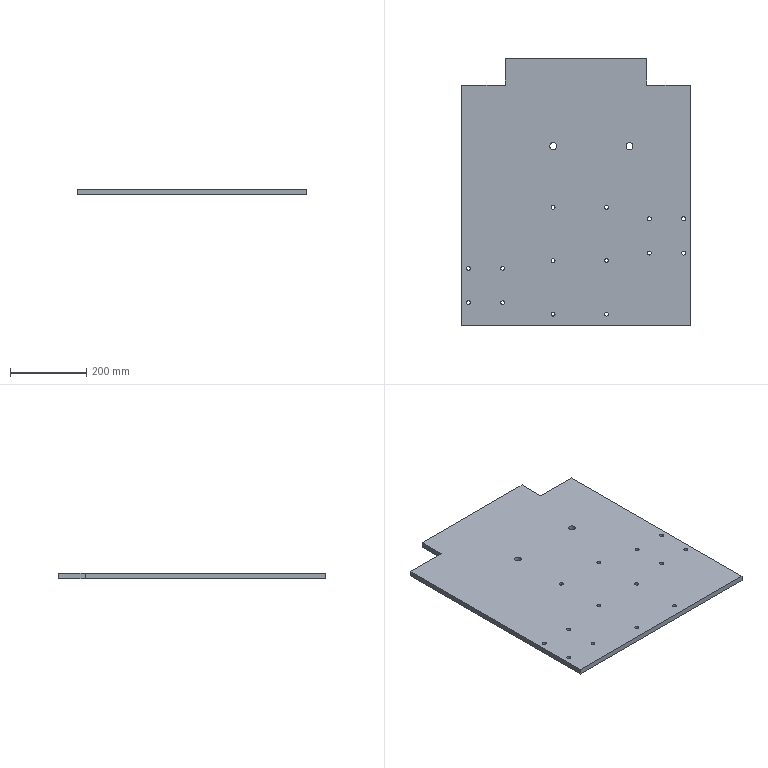Part | SolidWorks | features 3DProfileFeature 1, Extrusion 1, HoleWzd 1 | 1 solid | 42 faces | box 600 x 700 x 14 mm | volume 5631459 mm3 | cylinder 32 | plane 10 | commonest cylinder face diameters 10.2 x28 18 x4
STEP:
#1=CARTESIAN_POINT('',(12.9,150.,0.));
#2=VERTEX_POINT('',#1);
#3=CARTESIAN_POINT('',(23.1,150.,0.));
#4=VERTEX_POINT('',#3);
#5=CARTESIAN_POINT('',(18.,150.,0.));
#6=DIRECTION('',(0.,0.,1.));
#7=DIRECTION('',(1.,0.,0.));
#8=AXIS2_PLACEMENT_3D('',#5,#6,#7);
#9=CIRCLE('',#8,5.1);
#10=EDGE_CURVE('',#2,#4,#9,.T.);
#11=ORIENTED_EDGE('',*,*,#10,.F.);
#12=CARTESIAN_POINT('',(12.9,150.,14.));
#13=VERTEX_POINT('',#12);
#14=CARTESIAN_POINT('',(12.9,150.,14.));
#15=DIRECTION('',(0.,0.,1.));
#16=VECTOR('',#15,1000.);
#17=LINE('',#14,#16);
#18=EDGE_CURVE('',#2,#13,#17,.T.);
#19=ORIENTED_EDGE('',*,*,#18,.T.);
#20=CARTESIAN_POINT('',(23.1,150.,14.));
#21=VERTEX_POINT('',#20);
#22=CARTESIAN_POINT('',(18.,150.,14.));
#23=DIRECTION('',(0.,0.,1.));
#24=DIRECTION('',(1.,0.,0.));
#25=AXIS2_PLACEMENT_3D('',#22,#23,#24);
#26=CIRCLE('',#25,5.1);
#27=EDGE_CURVE('',#13,#21,#26,.T.);
#28=ORIENTED_EDGE('',*,*,#27,.T.);
#29=CARTESIAN_POINT('',(23.1,150.,14.));
#30=DIRECTION('',(0.,0.,1.));
#31=VECTOR('',#30,1000.);
#32=LINE('',#29,#31);
#33=EDGE_CURVE('',#4,#21,#32,.T.);
#34=ORIENTED_EDGE('',*,*,#33,.F.);
#35=EDGE_LOOP('',(#11,#19,#28,#34));
#36=FACE_OUTER_BOUND('',#35,.T.);
#37=CARTESIAN_POINT('',(18.,150.,14.));
#38=DIRECTION('',(0.,0.,1.));
#39=DIRECTION('',(1.,0.,0.));
#40=AXIS2_PLACEMENT_3D('',#37,#38,#39);
#41=CYLINDRICAL_SURFACE('',#40,5.1);
#42=ADVANCED_FACE('',(#36),#41,.F.);
#43=CARTESIAN_POINT('',(102.9,150.,0.));
#44=VERTEX_POINT('',#43);
#45=CARTESIAN_POINT('',(113.1,150.,0.));
#46=VERTEX_POINT('',#45);
#47=CARTESIAN_POINT('',(108.,150.,0.));
#48=DIRECTION('',(0.,0.,1.));
#49=DIRECTION('',(1.,0.,0.));
#50=AXIS2_PLACEMENT_3D('',#47,#48,#49);
#51=CIRCLE('',#50,5.1);
#52=EDGE_CURVE('',#44,#46,#51,.T.);
#53=ORIENTED_EDGE('',*,*,#52,.F.);
#54=CARTESIAN_POINT('',(102.9,150.,14.));
#55=VERTEX_POINT('',#54);
#56=CARTESIAN_POINT('',(102.9,150.,14.));
#57=DIRECTION('',(0.,0.,1.));
#58=VECTOR('',#57,1000.);
#59=LINE('',#56,#58);
#60=EDGE_CURVE('',#44,#55,#59,.T.);
#61=ORIENTED_EDGE('',*,*,#60,.T.);
#62=CARTESIAN_POINT('',(113.1,150.,14.));
#63=VERTEX_POINT('',#62);
#64=CARTESIAN_POINT('',(108.,150.,14.));
#65=DIRECTION('',(0.,0.,1.));
#66=DIRECTION('',(1.,0.,0.));
#67=AXIS2_PLACEMENT_3D('',#64,#65,#66);
#68=CIRCLE('',#67,5.1);
#69=EDGE_CURVE('',#55,#63,#68,.T.);
#70=ORIENTED_EDGE('',*,*,#69,.T.);
#71=CARTESIAN_POINT('',(113.1,150.,14.));
#72=DIRECTION('',(0.,0.,1.));
#73=VECTOR('',#72,1000.);
#74=LINE('',#71,#73);
#75=EDGE_CURVE('',#46,#63,#74,.T.);
#76=ORIENTED_EDGE('',*,*,#75,.F.);
#77=EDGE_LOOP('',(#53,#61,#70,#76));
#78=FACE_OUTER_BOUND('',#77,.T.);
#79=CARTESIAN_POINT('',(108.,150.,14.));
#80=DIRECTION('',(0.,0.,1.));
#81=DIRECTION('',(1.,0.,0.));
#82=AXIS2_PLACEMENT_3D('',#79,#80,#81);
#83=CYLINDRICAL_SURFACE('',#82,5.1);
#84=ADVANCED_FACE('',(#78),#83,.F.);
#85=CARTESIAN_POINT('',(12.9,60.,0.));
#86=VERTEX_POINT('',#85);
#87=CARTESIAN_POINT('',(23.1,60.,0.));
#88=VERTEX_POINT('',#87);
#89=CARTESIAN_POINT('',(18.,60.,0.));
#90=DIRECTION('',(0.,0.,1.));
#91=DIRECTION('',(1.,0.,0.));
#92=AXIS2_PLACEMENT_3D('',#89,#90,#91);
#93=CIRCLE('',#92,5.1);
#94=EDGE_CURVE('',#86,#88,#93,.T.);
#95=ORIENTED_EDGE('',*,*,#94,.F.);
#96=CARTESIAN_POINT('',(12.9,60.,14.));
#97=VERTEX_POINT('',#96);
#98=CARTESIAN_POINT('',(12.9,60.,14.));
#99=DIRECTION('',(0.,0.,1.));
#100=VECTOR('',#99,1000.);
#101=LINE('',#98,#100);
#102=EDGE_CURVE('',#86,#97,#101,.T.);
#103=ORIENTED_EDGE('',*,*,#102,.T.);
#104=CARTESIAN_POINT('',(23.1,60.,14.));
#105=VERTEX_POINT('',#104);
#106=CARTESIAN_POINT('',(18.,60.,14.));
#107=DIRECTION('',(0.,0.,1.));
#108=DIRECTION('',(1.,0.,0.));
#109=AXIS2_PLACEMENT_3D('',#106,#107,#108);
#110=CIRCLE('',#109,5.1);
#111=EDGE_CURVE('',#97,#105,#110,.T.);
#112=ORIENTED_EDGE('',*,*,#111,.T.);
#113=CARTESIAN_POINT('',(23.1,60.,14.));
#114=DIRECTION('',(0.,0.,1.));
#115=VECTOR('',#114,1000.);
#116=LINE('',#113,#115);
#117=EDGE_CURVE('',#88,#105,#116,.T.);
#118=ORIENTED_EDGE('',*,*,#117,.F.);
#119=EDGE_LOOP('',(#95,#103,#112,#118));
#120=FACE_OUTER_BOUND('',#119,.T.);
#121=CARTESIAN_POINT('',(18.,60.,14.));
#122=DIRECTION('',(0.,0.,1.));
#123=DIRECTION('',(1.,0.,0.));
#124=AXIS2_PLACEMENT_3D('',#121,#122,#123);
#125=CYLINDRICAL_SURFACE('',#124,5.1);
#126=ADVANCED_FACE('',(#120),#125,.F.);
#127=CARTESIAN_POINT('',(102.9,60.,0.));
#128=VERTEX_POINT('',#127);
#129=CARTESIAN_POINT('',(113.1,60.,0.));
#130=VERTEX_POINT('',#129);
#131=CARTESIAN_POINT('',(108.,60.,0.));
#132=DIRECTION('',(0.,0.,1.));
#133=DIRECTION('',(1.,0.,0.));
#134=AXIS2_PLACEMENT_3D('',#131,#132,#133);
#135=CIRCLE('',#134,5.1);
#136=EDGE_CURVE('',#128,#130,#135,.T.);
#137=ORIENTED_EDGE('',*,*,#136,.F.);
#138=CARTESIAN_POINT('',(102.9,60.,14.));
#139=VERTEX_POINT('',#138);
#140=CARTESIAN_POINT('',(102.9,60.,14.));
#141=DIRECTION('',(0.,0.,1.));
#142=VECTOR('',#141,1000.);
#143=LINE('',#140,#142);
#144=EDGE_CURVE('',#128,#139,#143,.T.);
#145=ORIENTED_EDGE('',*,*,#144,.T.);
#146=CARTESIAN_POINT('',(113.1,60.,14.));
#147=VERTEX_POINT('',#146);
#148=CARTESIAN_POINT('',(108.,60.,14.));
#149=DIRECTION('',(0.,0.,1.));
#150=DIRECTION('',(1.,0.,0.));
#151=AXIS2_PLACEMENT_3D('',#148,#149,#150);
#152=CIRCLE('',#151,5.1);
#153=EDGE_CURVE('',#139,#147,#152,.T.);
#154=ORIENTED_EDGE('',*,*,#153,.T.);
#155=CARTESIAN_POINT('',(113.1,60.,14.));
#156=DIRECTION('',(0.,0.,1.));
#157=VECTOR('',#156,1000.);
#158=LINE('',#155,#157);
#159=EDGE_CURVE('',#130,#147,#158,.T.);
#160=ORIENTED_EDGE('',*,*,#159,.F.);
#161=EDGE_LOOP('',(#137,#145,#154,#160));
#162=FACE_OUTER_BOUND('',#161,.T.);
#163=CARTESIAN_POINT('',(108.,60.,14.));
#164=DIRECTION('',(0.,0.,1.));
#165=DIRECTION('',(1.,0.,0.));
#166=AXIS2_PLACEMENT_3D('',#163,#164,#165);
#167=CYLINDRICAL_SURFACE('',#166,5.1);
#168=ADVANCED_FACE('',(#162),#167,.F.);
#169=CARTESIAN_POINT('',(486.9,280.,0.));
#170=VERTEX_POINT('',#169);
#171=CARTESIAN_POINT('',(497.1,280.,0.));
#172=VERTEX_POINT('',#171);
#173=CARTESIAN_POINT('',(492.,280.,0.));
#174=DIRECTION('',(0.,0.,1.));
#175=DIRECTION('',(1.,0.,0.));
#176=AXIS2_PLACEMENT_3D('',#173,#174,#175);
#177=CIRCLE('',#176,5.1);
#178=EDGE_CURVE('',#170,#172,#177,.T.);
#179=ORIENTED_EDGE('',*,*,#178,.F.);
#180=CARTESIAN_POINT('',(486.9,280.,14.));
#181=VERTEX_POINT('',#180);
#182=CARTESIAN_POINT('',(486.9,280.,14.));
#183=DIRECTION('',(0.,0.,1.));
#184=VECTOR('',#183,1000.);
#185=LINE('',#182,#184);
#186=EDGE_CURVE('',#170,#181,#185,.T.);
#187=ORIENTED_EDGE('',*,*,#186,.T.);
#188=CARTESIAN_POINT('',(497.1,280.,14.));
#189=VERTEX_POINT('',#188);
#190=CARTESIAN_POINT('',(492.,280.,14.));
#191=DIRECTION('',(0.,0.,1.));
#192=DIRECTION('',(1.,0.,0.));
#193=AXIS2_PLACEMENT_3D('',#190,#191,#192);
#194=CIRCLE('',#193,5.1);
#195=EDGE_CURVE('',#181,#189,#194,.T.);
#196=ORIENTED_EDGE('',*,*,#195,.T.);
#197=CARTESIAN_POINT('',(497.1,280.,14.));
#198=DIRECTION('',(0.,0.,1.));
#199=VECTOR('',#198,1000.);
#200=LINE('',#197,#199);
#201=EDGE_CURVE('',#172,#189,#200,.T.);
#202=ORIENTED_EDGE('',*,*,#201,.F.);
#203=EDGE_LOOP('',(#179,#187,#196,#202));
#204=FACE_OUTER_BOUND('',#203,.T.);
#205=CARTESIAN_POINT('',(492.,280.,14.));
#206=DIRECTION('',(0.,0.,1.));
#207=DIRECTION('',(1.,0.,0.));
#208=AXIS2_PLACEMENT_3D('',#205,#206,#207);
#209=CYLINDRICAL_SURFACE('',#208,5.1);
#210=ADVANCED_FACE('',(#204),#209,.F.);
#211=CARTESIAN_POINT('',(576.9,280.,0.));
#212=VERTEX_POINT('',#211);
#213=CARTESIAN_POINT('',(587.1,280.,0.));
#214=VERTEX_POINT('',#213);
#215=CARTESIAN_POINT('',(582.,280.,0.));
#216=DIRECTION('',(0.,0.,1.));
#217=DIRECTION('',(1.,0.,0.));
#218=AXIS2_PLACEMENT_3D('',#215,#216,#217);
#219=CIRCLE('',#218,5.1);
#220=EDGE_CURVE('',#212,#214,#219,.T.);
#221=ORIENTED_EDGE('',*,*,#220,.F.);
#222=CARTESIAN_POINT('',(576.9,280.,14.));
#223=VERTEX_POINT('',#222);
#224=CARTESIAN_POINT('',(576.9,280.,14.));
#225=DIRECTION('',(0.,0.,1.));
#226=VECTOR('',#225,1000.);
#227=LINE('',#224,#226);
#228=EDGE_CURVE('',#212,#223,#227,.T.);
#229=ORIENTED_EDGE('',*,*,#228,.T.);
#230=CARTESIAN_POINT('',(587.1,280.,14.));
#231=VERTEX_POINT('',#230);
#232=CARTESIAN_POINT('',(582.,280.,14.));
#233=DIRECTION('',(0.,0.,1.));
#234=DIRECTION('',(1.,0.,0.));
#235=AXIS2_PLACEMENT_3D('',#232,#233,#234);
#236=CIRCLE('',#235,5.1);
#237=EDGE_CURVE('',#223,#231,#236,.T.);
#238=ORIENTED_EDGE('',*,*,#237,.T.);
#239=CARTESIAN_POINT('',(587.1,280.,14.));
#240=DIRECTION('',(0.,0.,1.));
#241=VECTOR('',#240,1000.);
#242=LINE('',#239,#241);
#243=EDGE_CURVE('',#214,#231,#242,.T.);
#244=ORIENTED_EDGE('',*,*,#243,.F.);
#245=EDGE_LOOP('',(#221,#229,#238,#244));
#246=FACE_OUTER_BOUND('',#245,.T.);
#247=CARTESIAN_POINT('',(582.,280.,14.));
#248=DIRECTION('',(0.,0.,1.));
#249=DIRECTION('',(1.,0.,0.));
#250=AXIS2_PLACEMENT_3D('',#247,#248,#249);
#251=CYLINDRICAL_SURFACE('',#250,5.1);
#252=ADVANCED_FACE('',(#246),#251,.F.);
#253=CARTESIAN_POINT('',(486.9,190.,0.));
#254=VERTEX_POINT('',#253);
#255=CARTESIAN_POINT('',(497.1,190.,0.));
#256=VERTEX_POINT('',#255);
#257=CARTESIAN_POINT('',(492.,190.,0.));
#258=DIRECTION('',(0.,0.,1.));
#259=DIRECTION('',(1.,0.,0.));
#260=AXIS2_PLACEMENT_3D('',#257,#258,#259);
#261=CIRCLE('',#260,5.1);
#262=EDGE_CURVE('',#254,#256,#261,.T.);
#263=ORIENTED_EDGE('',*,*,#262,.F.);
#264=CARTESIAN_POINT('',(486.9,190.,14.));
#265=VERTEX_POINT('',#264);
#266=CARTESIAN_POINT('',(486.9,190.,14.));
#267=DIRECTION('',(0.,0.,1.));
#268=VECTOR('',#267,1000.);
#269=LINE('',#266,#268);
#270=EDGE_CURVE('',#254,#265,#269,.T.);
#271=ORIENTED_EDGE('',*,*,#270,.T.);
#272=CARTESIAN_POINT('',(497.1,190.,14.));
#273=VERTEX_POINT('',#272);
#274=CARTESIAN_POINT('',(492.,190.,14.));
#275=DIRECTION('',(0.,0.,1.));
#276=DIRECTION('',(1.,0.,0.));
#277=AXIS2_PLACEMENT_3D('',#274,#275,#276);
#278=CIRCLE('',#277,5.1);
#279=EDGE_CURVE('',#265,#273,#278,.T.);
#280=ORIENTED_EDGE('',*,*,#279,.T.);
#281=CARTESIAN_POINT('',(497.1,190.,14.));
#282=DIRECTION('',(0.,0.,1.));
#283=VECTOR('',#282,1000.);
#284=LINE('',#281,#283);
#285=EDGE_CURVE('',#256,#273,#284,.T.);
#286=ORIENTED_EDGE('',*,*,#285,.F.);
#287=EDGE_LOOP('',(#263,#271,#280,#286));
#288=FACE_OUTER_BOUND('',#287,.T.);
#289=CARTESIAN_POINT('',(492.,190.,14.));
#290=DIRECTION('',(0.,0.,1.));
#291=DIRECTION('',(1.,0.,0.));
#292=AXIS2_PLACEMENT_3D('',#289,#290,#291);
#293=CYLINDRICAL_SURFACE('',#292,5.1);
#294=ADVANCED_FACE('',(#288),#293,.F.);
#295=CARTESIAN_POINT('',(576.9,190.,0.));
#296=VERTEX_POINT('',#295);
#297=CARTESIAN_POINT('',(587.1,190.,0.));
#298=VERTEX_POINT('',#297);
#299=CARTESIAN_POINT('',(582.,190.,0.));
#300=DIRECTION('',(0.,0.,1.));
#301=DIRECTION('',(1.,0.,0.));
#302=AXIS2_PLACEMENT_3D('',#299,#300,#301);
#303=CIRCLE('',#302,5.1);
#304=EDGE_CURVE('',#296,#298,#303,.T.);
#305=ORIENTED_EDGE('',*,*,#304,.F.);
#306=CARTESIAN_POINT('',(576.9,190.,14.));
#307=VERTEX_POINT('',#306);
#308=CARTESIAN_POINT('',(576.9,190.,14.));
#309=DIRECTION('',(0.,0.,1.));
#310=VECTOR('',#309,1000.);
#311=LINE('',#308,#310);
#312=EDGE_CURVE('',#296,#307,#311,.T.);
#313=ORIENTED_EDGE('',*,*,#312,.T.);
#314=CARTESIAN_POINT('',(587.1,190.,14.));
#315=VERTEX_POINT('',#314);
#316=CARTESIAN_POINT('',(582.,190.,14.));
#317=DIRECTION('',(0.,0.,1.));
#318=DIRECTION('',(1.,0.,0.));
#319=AXIS2_PLACEMENT_3D('',#316,#317,#318);
#320=CIRCLE('',#319,5.1);
#321=EDGE_CURVE('',#307,#315,#320,.T.);
#322=ORIENTED_EDGE('',*,*,#321,.T.);
#323=CARTESIAN_POINT('',(587.1,190.,14.));
#324=DIRECTION('',(0.,0.,1.));
#325=VECTOR('',#324,1000.);
#326=LINE('',#323,#325);
#327=EDGE_CURVE('',#298,#315,#326,.T.);
#328=ORIENTED_EDGE('',*,*,#327,.F.);
#329=EDGE_LOOP('',(#305,#313,#322,#328));
#330=FACE_OUTER_BOUND('',#329,.T.);
#331=CARTESIAN_POINT('',(582.,190.,14.));
#332=DIRECTION('',(0.,0.,1.));
#333=DIRECTION('',(1.,0.,0.));
#334=AXIS2_PLACEMENT_3D('',#331,#332,#333);
#335=CYLINDRICAL_SURFACE('',#334,5.1);
#336=ADVANCED_FACE('',(#330),#335,.F.);
#337=CARTESIAN_POINT('',(234.9,310.,0.));
#338=VERTEX_POINT('',#337);
#339=CARTESIAN_POINT('',(245.1,310.,0.));
#340=VERTEX_POINT('',#339);
#341=CARTESIAN_POINT('',(240.,310.,0.));
#342=DIRECTION('',(0.,0.,1.));
#343=DIRECTION('',(1.,0.,0.));
#344=AXIS2_PLACEMENT_3D('',#341,#342,#343);
#345=CIRCLE('',#344,5.1);
#346=EDGE_CURVE('',#338,#340,#345,.T.);
#347=ORIENTED_EDGE('',*,*,#346,.F.);
#348=CARTESIAN_POINT('',(234.9,310.,14.));
#349=VERTEX_POINT('',#348);
#350=CARTESIAN_POINT('',(234.9,310.,14.));
#351=DIRECTION('',(0.,0.,1.));
#352=VECTOR('',#351,1000.);
#353=LINE('',#350,#352);
#354=EDGE_CURVE('',#338,#349,#353,.T.);
#355=ORIENTED_EDGE('',*,*,#354,.T.);
#356=CARTESIAN_POINT('',(245.1,310.,14.));
#357=VERTEX_POINT('',#356);
#358=CARTESIAN_POINT('',(240.,310.,14.));
#359=DIRECTION('',(0.,0.,1.));
#360=DIRECTION('',(1.,0.,0.));
#361=AXIS2_PLACEMENT_3D('',#358,#359,#360);
#362=CIRCLE('',#361,5.1);
#363=EDGE_CURVE('',#349,#357,#362,.T.);
#364=ORIENTED_EDGE('',*,*,#363,.T.);
#365=CARTESIAN_POINT('',(245.1,310.,14.));
#366=DIRECTION('',(0.,0.,1.));
#367=VECTOR('',#366,1000.);
#368=LINE('',#365,#367);
#369=EDGE_CURVE('',#340,#357,#368,.T.);
#370=ORIENTED_EDGE('',*,*,#369,.F.);
#371=EDGE_LOOP('',(#347,#355,#364,#370));
#372=FACE_OUTER_BOUND('',#371,.T.);
#373=CARTESIAN_POINT('',(240.,310.,14.));
#374=DIRECTION('',(0.,0.,1.));
#375=DIRECTION('',(1.,0.,0.));
#376=AXIS2_PLACEMENT_3D('',#373,#374,#375);
#377=CYLINDRICAL_SURFACE('',#376,5.1);
#378=ADVANCED_FACE('',(#372),#377,.F.);
#379=CARTESIAN_POINT('',(374.9,310.,0.));
#380=VERTEX_POINT('',#379);
#381=CARTESIAN_POINT('',(385.1,310.,0.));
#382=VERTEX_POINT('',#381);
#383=CARTESIAN_POINT('',(380.,310.,0.));
#384=DIRECTION('',(0.,0.,1.));
#385=DIRECTION('',(1.,0.,0.));
#386=AXIS2_PLACEMENT_3D('',#383,#384,#385);
#387=CIRCLE('',#386,5.1);
#388=EDGE_CURVE('',#380,#382,#387,.T.);
#389=ORIENTED_EDGE('',*,*,#388,.F.);
#390=CARTESIAN_POINT('',(374.9,310.,14.));
#391=VERTEX_POINT('',#390);
#392=CARTESIAN_POINT('',(374.9,310.,14.));
#393=DIRECTION('',(0.,0.,1.));
#394=VECTOR('',#393,1000.);
#395=LINE('',#392,#394);
#396=EDGE_CURVE('',#380,#391,#395,.T.);
#397=ORIENTED_EDGE('',*,*,#396,.T.);
#398=CARTESIAN_POINT('',(385.1,310.,14.));
#399=VERTEX_POINT('',#398);
#400=CARTESIAN_POINT('',(380.,310.,14.));
#401=DIRECTION('',(0.,0.,1.));
#402=DIRECTION('',(1.,0.,0.));
#403=AXIS2_PLACEMENT_3D('',#400,#401,#402);
#404=CIRCLE('',#403,5.1);
#405=EDGE_CURVE('',#391,#399,#404,.T.);
#406=ORIENTED_EDGE('',*,*,#405,.T.);
#407=CARTESIAN_POINT('',(385.1,310.,14.));
#408=DIRECTION('',(0.,0.,1.));
#409=VECTOR('',#408,1000.);
#410=LINE('',#407,#409);
#411=EDGE_CURVE('',#382,#399,#410,.T.);
#412=ORIENTED_EDGE('',*,*,#411,.F.);
#413=EDGE_LOOP('',(#389,#397,#406,#412));
#414=FACE_OUTER_BOUND('',#413,.T.);
#415=CARTESIAN_POINT('',(380.,310.,14.));
#416=DIRECTION('',(0.,0.,1.));
#417=DIRECTION('',(1.,0.,0.));
#418=AXIS2_PLACEMENT_3D('',#415,#416,#417);
#419=CYLINDRICAL_SURFACE('',#418,5.1);
#420=ADVANCED_FACE('',(#414),#419,.F.);
#421=CARTESIAN_POINT('',(234.9,170.,0.));
#422=VERTEX_POINT('',#421);
#423=CARTESIAN_POINT('',(245.1,170.,0.));
#424=VERTEX_POINT('',#423);
#425=CARTESIAN_POINT('',(240.,170.,0.));
#426=DIRECTION('',(0.,0.,1.));
#427=DIRECTION('',(1.,0.,0.));
#428=AXIS2_PLACEMENT_3D('',#425,#426,#427);
#429=CIRCLE('',#428,5.1);
#430=EDGE_CURVE('',#422,#424,#429,.T.);
#431=ORIENTED_EDGE('',*,*,#430,.F.);
#432=CARTESIAN_POINT('',(234.9,170.,14.));
#433=VERTEX_POINT('',#432);
#434=CARTESIAN_POINT('',(234.9,170.,14.));
#435=DIRECTION('',(0.,0.,1.));
#436=VECTOR('',#435,1000.);
#437=LINE('',#434,#436);
#438=EDGE_CURVE('',#422,#433,#437,.T.);
#439=ORIENTED_EDGE('',*,*,#438,.T.);
#440=CARTESIAN_POINT('',(245.1,170.,14.));
#441=VERTEX_POINT('',#440);
#442=CARTESIAN_POINT('',(240.,170.,14.));
#443=DIRECTION('',(0.,0.,1.));
#444=DIRECTION('',(1.,0.,0.));
#445=AXIS2_PLACEMENT_3D('',#442,#443,#444);
#446=CIRCLE('',#445,5.1);
#447=EDGE_CURVE('',#433,#441,#446,.T.);
#448=ORIENTED_EDGE('',*,*,#447,.T.);
#449=CARTESIAN_POINT('',(245.1,170.,14.));
#450=DIRECTION('',(0.,0.,1.));
#451=VECTOR('',#450,1000.);
#452=LINE('',#449,#451);
#453=EDGE_CURVE('',#424,#441,#452,.T.);
#454=ORIENTED_EDGE('',*,*,#453,.F.);
#455=EDGE_LOOP('',(#431,#439,#448,#454));
#456=FACE_OUTER_BOUND('',#455,.T.);
#457=CARTESIAN_POINT('',(240.,170.,14.));
#458=DIRECTION('',(0.,0.,1.));
#459=DIRECTION('',(1.,0.,0.));
#460=AXIS2_PLACEMENT_3D('',#457,#458,#459);
#461=CYLINDRICAL_SURFACE('',#460,5.1);
#462=ADVANCED_FACE('',(#456),#461,.F.);
#463=CARTESIAN_POINT('',(374.9,170.,0.));
#464=VERTEX_POINT('',#463);
#465=CARTESIAN_POINT('',(385.1,170.,0.));
#466=VERTEX_POINT('',#465);
#467=CARTESIAN_POINT('',(380.,170.,0.));
#468=DIRECTION('',(0.,0.,1.));
#469=DIRECTION('',(1.,0.,0.));
#470=AXIS2_PLACEMENT_3D('',#467,#468,#469);
#471=CIRCLE('',#470,5.1);
#472=EDGE_CURVE('',#464,#466,#471,.T.);
#473=ORIENTED_EDGE('',*,*,#472,.F.);
#474=CARTESIAN_POINT('',(374.9,170.,14.));
#475=VERTEX_POINT('',#474);
#476=CARTESIAN_POINT('',(374.9,170.,14.));
#477=DIRECTION('',(0.,0.,1.));
#478=VECTOR('',#477,1000.);
#479=LINE('',#476,#478);
#480=EDGE_CURVE('',#464,#475,#479,.T.);
#481=ORIENTED_EDGE('',*,*,#480,.T.);
#482=CARTESIAN_POINT('',(385.1,170.,14.));
#483=VERTEX_POINT('',#482);
#484=CARTESIAN_POINT('',(380.,170.,14.));
#485=DIRECTION('',(0.,0.,1.));
#486=DIRECTION('',(1.,0.,0.));
#487=AXIS2_PLACEMENT_3D('',#484,#485,#486);
#488=CIRCLE('',#487,5.1);
#489=EDGE_CURVE('',#475,#483,#488,.T.);
#490=ORIENTED_EDGE('',*,*,#489,.T.);
#491=CARTESIAN_POINT('',(385.1,170.,14.));
#492=DIRECTION('',(0.,0.,1.));
#493=VECTOR('',#492,1000.);
#494=LINE('',#491,#493);
#495=EDGE_CURVE('',#466,#483,#494,.T.);
#496=ORIENTED_EDGE('',*,*,#495,.F.);
#497=EDGE_LOOP('',(#473,#481,#490,#496));
#498=FACE_OUTER_BOUND('',#497,.T.);
#499=CARTESIAN_POINT('',(380.,170.,14.));
#500=DIRECTION('',(0.,0.,1.));
#501=DIRECTION('',(1.,0.,0.));
#502=AXIS2_PLACEMENT_3D('',#499,#500,#501);
#503=CYLINDRICAL_SURFACE('',#502,5.1);
#504=ADVANCED_FACE('',(#498),#503,.F.);
#505=CARTESIAN_POINT('',(234.9,30.,0.));
#506=VERTEX_POINT('',#505);
#507=CARTESIAN_POINT('',(245.1,30.,0.));
#508=VERTEX_POINT('',#507);
#509=CARTESIAN_POINT('',(240.,30.,0.));
#510=DIRECTION('',(0.,0.,1.));
#511=DIRECTION('',(1.,0.,0.));
#512=AXIS2_PLACEMENT_3D('',#509,#510,#511);
#513=CIRCLE('',#512,5.1);
#514=EDGE_CURVE('',#506,#508,#513,.T.);
#515=ORIENTED_EDGE('',*,*,#514,.F.);
#516=CARTESIAN_POINT('',(234.9,30.,14.));
#517=VERTEX_POINT('',#516);
#518=CARTESIAN_POINT('',(234.9,30.,14.));
#519=DIRECTION('',(0.,0.,1.));
#520=VECTOR('',#519,1000.);
#521=LINE('',#518,#520);
#522=EDGE_CURVE('',#506,#517,#521,.T.);
#523=ORIENTED_EDGE('',*,*,#522,.T.);
#524=CARTESIAN_POINT('',(245.1,30.,14.));
#525=VERTEX_POINT('',#524);
#526=CARTESIAN_POINT('',(240.,30.,14.));
#527=DIRECTION('',(0.,0.,1.));
#528=DIRECTION('',(1.,0.,0.));
#529=AXIS2_PLACEMENT_3D('',#526,#527,#528);
#530=CIRCLE('',#529,5.1);
#531=EDGE_CURVE('',#517,#525,#530,.T.);
#532=ORIENTED_EDGE('',*,*,#531,.T.);
#533=CARTESIAN_POINT('',(245.1,30.,14.));
#534=DIRECTION('',(0.,0.,1.));
#535=VECTOR('',#534,1000.);
#536=LINE('',#533,#535);
#537=EDGE_CURVE('',#508,#525,#536,.T.);
#538=ORIENTED_EDGE('',*,*,#537,.F.);
#539=EDGE_LOOP('',(#515,#523,#532,#538));
#540=FACE_OUTER_BOUND('',#539,.T.);
#541=CARTESIAN_POINT('',(240.,30.,14.));
#542=DIRECTION('',(0.,0.,1.));
#543=DIRECTION('',(1.,0.,0.));
#544=AXIS2_PLACEMENT_3D('',#541,#542,#543);
#545=CYLINDRICAL_SURFACE('',#544,5.1);
#546=ADVANCED_FACE('',(#540),#545,.F.);
#547=CARTESIAN_POINT('',(374.9,30.,0.));
#548=VERTEX_POINT('',#547);
#549=CARTESIAN_POINT('',(385.1,30.,0.));
#550=VERTEX_POINT('',#549);
#551=CARTESIAN_POINT('',(380.,30.,0.));
#552=DIRECTION('',(0.,0.,1.));
#553=DIRECTION('',(1.,0.,0.));
#554=AXIS2_PLACEMENT_3D('',#551,#552,#553);
#555=CIRCLE('',#554,5.1);
#556=EDGE_CURVE('',#548,#550,#555,.T.);
#557=ORIENTED_EDGE('',*,*,#556,.F.);
#558=CARTESIAN_POINT('',(374.9,30.,14.));
#559=VERTEX_POINT('',#558);
#560=CARTESIAN_POINT('',(374.9,30.,14.));
#561=DIRECTION('',(0.,0.,1.));
#562=VECTOR('',#561,1000.);
#563=LINE('',#560,#562);
#564=EDGE_CURVE('',#548,#559,#563,.T.);
#565=ORIENTED_EDGE('',*,*,#564,.T.);
#566=CARTESIAN_POINT('',(385.1,30.,14.));
#567=VERTEX_POINT('',#566);
#568=CARTESIAN_POINT('',(380.,30.,14.));
#569=DIRECTION('',(0.,0.,1.));
#570=DIRECTION('',(1.,0.,0.));
#571=AXIS2_PLACEMENT_3D('',#568,#569,#570);
#572=CIRCLE('',#571,5.1);
#573=EDGE_CURVE('',#559,#567,#572,.T.);
#574=ORIENTED_EDGE('',*,*,#573,.T.);
#575=CARTESIAN_POINT('',(385.1,30.,14.));
#576=DIRECTION('',(0.,0.,1.));
#577=VECTOR('',#576,1000.);
#578=LINE('',#575,#577);
#579=EDGE_CURVE('',#550,#567,#578,.T.);
#580=ORIENTED_EDGE('',*,*,#579,.F.);
#581=EDGE_LOOP('',(#557,#565,#574,#580));
#582=FACE_OUTER_BOUND('',#581,.T.);
#583=CARTESIAN_POINT('',(380.,30.,14.));
#584=DIRECTION('',(0.,0.,1.));
#585=DIRECTION('',(1.,0.,0.));
#586=AXIS2_PLACEMENT_3D('',#583,#584,#585);
#587=CYLINDRICAL_SURFACE('',#586,5.1);
#588=ADVANCED_FACE('',(#582),#587,.F.);
#589=CARTESIAN_POINT('',(231.,470.,14.));
#590=VERTEX_POINT('',#589);
#591=CARTESIAN_POINT('',(249.,470.,14.));
#592=VERTEX_POINT('',#591);
#593=CARTESIAN_POINT('',(240.,470.,14.));
#594=DIRECTION('',(0.,0.,1.));
#595=DIRECTION('',(1.,0.,0.));
#596=AXIS2_PLACEMENT_3D('',#593,#594,#595);
#597=CIRCLE('',#596,9.);
#598=EDGE_CURVE('',#590,#592,#597,.T.);
#599=ORIENTED_EDGE('',*,*,#598,.T.);
#600=CARTESIAN_POINT('',(249.,470.,0.));
#601=VERTEX_POINT('',#600);
#602=CARTESIAN_POINT('',(249.,470.,14.));
#603=DIRECTION('',(0.,0.,-1.));
#604=VECTOR('',#603,1000.);
#605=LINE('',#602,#604);
#606=EDGE_CURVE('',#592,#601,#605,.T.);
#607=ORIENTED_EDGE('',*,*,#606,.T.);
#608=CARTESIAN_POINT('',(231.,470.,0.));
#609=VERTEX_POINT('',#608);
#610=CARTESIAN_POINT('',(240.,470.,0.));
#611=DIRECTION('',(0.,0.,1.));
#612=DIRECTION('',(1.,0.,0.));
#613=AXIS2_PLACEMENT_3D('',#610,#611,#612);
#614=CIRCLE('',#613,9.);
#615=EDGE_CURVE('',#609,#601,#614,.T.);
#616=ORIENTED_EDGE('',*,*,#615,.F.);
#617=CARTESIAN_POINT('',(231.,470.,14.));
#618=DIRECTION('',(0.,0.,-1.));
#619=VECTOR('',#618,1000.);
#620=LINE('',#617,#619);
#621=EDGE_CURVE('',#590,#609,#620,.T.);
#622=ORIENTED_EDGE('',*,*,#621,.F.);
#623=EDGE_LOOP('',(#599,#607,#616,#622));
#624=FACE_OUTER_BOUND('',#623,.T.);
#625=CARTESIAN_POINT('',(240.,470.,14.));
#626=DIRECTION('',(0.,0.,-1.));
#627=DIRECTION('',(-1.,0.,0.));
#628=AXIS2_PLACEMENT_3D('',#625,#626,#627);
#629=CYLINDRICAL_SURFACE('',#628,9.);
#630=ADVANCED_FACE('',(#624),#629,.F.);
#631=CARTESIAN_POINT('',(431.,470.,14.));
#632=VERTEX_POINT('',#631);
#633=CARTESIAN_POINT('',(449.,470.,14.));
#634=VERTEX_POINT('',#633);
#635=CARTESIAN_POINT('',(440.,470.,14.));
#636=DIRECTION('',(0.,0.,1.));
#637=DIRECTION('',(1.,0.,0.));
#638=AXIS2_PLACEMENT_3D('',#635,#636,#637);
#639=CIRCLE('',#638,9.);
#640=EDGE_CURVE('',#632,#634,#639,.T.);
#641=ORIENTED_EDGE('',*,*,#640,.T.);
#642=CARTESIAN_POINT('',(449.,470.,0.));
#643=VERTEX_POINT('',#642);
#644=CARTESIAN_POINT('',(449.,470.,14.));
#645=DIRECTION('',(0.,0.,-1.));
#646=VECTOR('',#645,1000.);
#647=LINE('',#644,#646);
#648=EDGE_CURVE('',#634,#643,#647,.T.);
#649=ORIENTED_EDGE('',*,*,#648,.T.);
#650=CARTESIAN_POINT('',(431.,470.,0.));
#651=VERTEX_POINT('',#650);
#652=CARTESIAN_POINT('',(440.,470.,0.));
#653=DIRECTION('',(0.,0.,1.));
#654=DIRECTION('',(1.,0.,0.));
#655=AXIS2_PLACEMENT_3D('',#652,#653,#654);
#656=CIRCLE('',#655,9.);
#657=EDGE_CURVE('',#651,#643,#656,.T.);
#658=ORIENTED_EDGE('',*,*,#657,.F.);
#659=CARTESIAN_POINT('',(431.,470.,14.));
#660=DIRECTION('',(0.,0.,-1.));
#661=VECTOR('',#660,1000.);
#662=LINE('',#659,#661);
#663=EDGE_CURVE('',#632,#651,#662,.T.);
#664=ORIENTED_EDGE('',*,*,#663,.F.);
#665=EDGE_LOOP('',(#641,#649,#658,#664));
#666=FACE_OUTER_BOUND('',#665,.T.);
#667=CARTESIAN_POINT('',(440.,470.,14.));
#668=DIRECTION('',(0.,0.,-1.));
#669=DIRECTION('',(-1.,0.,0.));
#670=AXIS2_PLACEMENT_3D('',#667,#668,#669);
#671=CYLINDRICAL_SURFACE('',#670,9.);
#672=ADVANCED_FACE('',(#666),#671,.F.);
#673=CARTESIAN_POINT('',(18.,150.,14.));
#674=DIRECTION('',(0.,0.,1.));
#675=DIRECTION('',(1.,0.,0.));
#676=AXIS2_PLACEMENT_3D('',#673,#674,#675);
#677=CIRCLE('',#676,5.1);
#678=EDGE_CURVE('',#21,#13,#677,.T.);
#679=ORIENTED_EDGE('',*,*,#678,.F.);
#680=ORIENTED_EDGE('',*,*,#27,.F.);
#681=EDGE_LOOP('',(#679,#680));
#682=FACE_BOUND('',#681,.T.);
#683=CARTESIAN_POINT('',(108.,150.,14.));
#684=DIRECTION('',(0.,0.,1.));
#685=DIRECTION('',(1.,0.,0.));
#686=AXIS2_PLACEMENT_3D('',#683,#684,#685);
#687=CIRCLE('',#686,5.1);
#688=EDGE_CURVE('',#63,#55,#687,.T.);
#689=ORIENTED_EDGE('',*,*,#688,.F.);
#690=ORIENTED_EDGE('',*,*,#69,.F.);
#691=EDGE_LOOP('',(#689,#690));
#692=FACE_BOUND('',#691,.T.);
#693=CARTESIAN_POINT('',(18.,60.,14.));
#694=DIRECTION('',(0.,0.,1.));
#695=DIRECTION('',(1.,0.,0.));
#696=AXIS2_PLACEMENT_3D('',#693,#694,#695);
#697=CIRCLE('',#696,5.1);
#698=EDGE_CURVE('',#105,#97,#697,.T.);
#699=ORIENTED_EDGE('',*,*,#698,.F.);
#700=ORIENTED_EDGE('',*,*,#111,.F.);
#701=EDGE_LOOP('',(#699,#700));
#702=FACE_BOUND('',#701,.T.);
#703=CARTESIAN_POINT('',(108.,60.,14.));
#704=DIRECTION('',(0.,0.,1.));
#705=DIRECTION('',(1.,0.,0.));
#706=AXIS2_PLACEMENT_3D('',#703,#704,#705);
#707=CIRCLE('',#706,5.1);
#708=EDGE_CURVE('',#147,#139,#707,.T.);
#709=ORIENTED_EDGE('',*,*,#708,.F.);
#710=ORIENTED_EDGE('',*,*,#153,.F.);
#711=EDGE_LOOP('',(#709,#710));
#712=FACE_BOUND('',#711,.T.);
#713=CARTESIAN_POINT('',(492.,280.,14.));
#714=DIRECTION('',(0.,0.,1.));
#715=DIRECTION('',(1.,0.,0.));
#716=AXIS2_PLACEMENT_3D('',#713,#714,#715);
#717=CIRCLE('',#716,5.1);
#718=EDGE_CURVE('',#189,#181,#717,.T.);
#719=ORIENTED_EDGE('',*,*,#718,.F.);
#720=ORIENTED_EDGE('',*,*,#195,.F.);
#721=EDGE_LOOP('',(#719,#720));
#722=FACE_BOUND('',#721,.T.);
#723=CARTESIAN_POINT('',(582.,280.,14.));
#724=DIRECTION('',(0.,0.,1.));
#725=DIRECTION('',(1.,0.,0.));
#726=AXIS2_PLACEMENT_3D('',#723,#724,#725);
#727=CIRCLE('',#726,5.1);
#728=EDGE_CURVE('',#231,#223,#727,.T.);
#729=ORIENTED_EDGE('',*,*,#728,.F.);
#730=ORIENTED_EDGE('',*,*,#237,.F.);
#731=EDGE_LOOP('',(#729,#730));
#732=FACE_BOUND('',#731,.T.);
#733=CARTESIAN_POINT('',(492.,190.,14.));
#734=DIRECTION('',(0.,0.,1.));
#735=DIRECTION('',(1.,0.,0.));
#736=AXIS2_PLACEMENT_3D('',#733,#734,#735);
#737=CIRCLE('',#736,5.1);
#738=EDGE_CURVE('',#273,#265,#737,.T.);
#739=ORIENTED_EDGE('',*,*,#738,.F.);
#740=ORIENTED_EDGE('',*,*,#279,.F.);
#741=EDGE_LOOP('',(#739,#740));
#742=FACE_BOUND('',#741,.T.);
#743=CARTESIAN_POINT('',(582.,190.,14.));
#744=DIRECTION('',(0.,0.,1.));
#745=DIRECTION('',(1.,0.,0.));
#746=AXIS2_PLACEMENT_3D('',#743,#744,#745);
#747=CIRCLE('',#746,5.1);
#748=EDGE_CURVE('',#315,#307,#747,.T.);
#749=ORIENTED_EDGE('',*,*,#748,.F.);
#750=ORIENTED_EDGE('',*,*,#321,.F.);
#751=EDGE_LOOP('',(#749,#750));
#752=FACE_BOUND('',#751,.T.);
#753=CARTESIAN_POINT('',(240.,310.,14.));
#754=DIRECTION('',(0.,0.,1.));
#755=DIRECTION('',(1.,0.,0.));
#756=AXIS2_PLACEMENT_3D('',#753,#754,#755);
#757=CIRCLE('',#756,5.1);
#758=EDGE_CURVE('',#357,#349,#757,.T.);
#759=ORIENTED_EDGE('',*,*,#758,.F.);
#760=ORIENTED_EDGE('',*,*,#363,.F.);
#761=EDGE_LOOP('',(#759,#760));
#762=FACE_BOUND('',#761,.T.);
#763=CARTESIAN_POINT('',(380.,310.,14.));
#764=DIRECTION('',(0.,0.,1.));
#765=DIRECTION('',(1.,0.,0.));
#766=AXIS2_PLACEMENT_3D('',#763,#764,#765);
#767=CIRCLE('',#766,5.1);
#768=EDGE_CURVE('',#399,#391,#767,.T.);
#769=ORIENTED_EDGE('',*,*,#768,.F.);
#770=ORIENTED_EDGE('',*,*,#405,.F.);
#771=EDGE_LOOP('',(#769,#770));
#772=FACE_BOUND('',#771,.T.);
#773=CARTESIAN_POINT('',(240.,170.,14.));
#774=DIRECTION('',(0.,0.,1.));
#775=DIRECTION('',(1.,0.,0.));
#776=AXIS2_PLACEMENT_3D('',#773,#774,#775);
#777=CIRCLE('',#776,5.1);
#778=EDGE_CURVE('',#441,#433,#777,.T.);
#779=ORIENTED_EDGE('',*,*,#778,.F.);
#780=ORIENTED_EDGE('',*,*,#447,.F.);
#781=EDGE_LOOP('',(#779,#780));
#782=FACE_BOUND('',#781,.T.);
#783=CARTESIAN_POINT('',(380.,170.,14.));
#784=DIRECTION('',(0.,0.,1.));
#785=DIRECTION('',(1.,0.,0.));
#786=AXIS2_PLACEMENT_3D('',#783,#784,#785);
#787=CIRCLE('',#786,5.1);
#788=EDGE_CURVE('',#483,#475,#787,.T.);
#789=ORIENTED_EDGE('',*,*,#788,.F.);
#790=ORIENTED_EDGE('',*,*,#489,.F.);
#791=EDGE_LOOP('',(#789,#790));
#792=FACE_BOUND('',#791,.T.);
#793=CARTESIAN_POINT('',(240.,30.,14.));
#794=DIRECTION('',(0.,0.,1.));
#795=DIRECTION('',(1.,0.,0.));
#796=AXIS2_PLACEMENT_3D('',#793,#794,#795);
#797=CIRCLE('',#796,5.1);
#798=EDGE_CURVE('',#525,#517,#797,.T.);
#799=ORIENTED_EDGE('',*,*,#798,.F.);
#800=ORIENTED_EDGE('',*,*,#531,.F.);
#801=EDGE_LOOP('',(#799,#800));
#802=FACE_BOUND('',#801,.T.);
#803=CARTESIAN_POINT('',(380.,30.,14.));
#804=DIRECTION('',(0.,0.,1.));
#805=DIRECTION('',(1.,0.,0.));
#806=AXIS2_PLACEMENT_3D('',#803,#804,#805);
#807=CIRCLE('',#806,5.1);
#808=EDGE_CURVE('',#567,#559,#807,.T.);
#809=ORIENTED_EDGE('',*,*,#808,.F.);
#810=ORIENTED_EDGE('',*,*,#573,.F.);
#811=EDGE_LOOP('',(#809,#810));
#812=FACE_BOUND('',#811,.T.);
#813=ORIENTED_EDGE('',*,*,#640,.F.);
#814=CARTESIAN_POINT('',(440.,470.,14.));
#815=DIRECTION('',(0.,0.,1.));
#816=DIRECTION('',(1.,0.,0.));
#817=AXIS2_PLACEMENT_3D('',#814,#815,#816);
#818=CIRCLE('',#817,9.);
#819=EDGE_CURVE('',#634,#632,#818,.T.);
#820=ORIENTED_EDGE('',*,*,#819,.F.);
#821=EDGE_LOOP('',(#813,#820));
#822=FACE_BOUND('',#821,.T.);
#823=CARTESIAN_POINT('',(0.,630.,14.));
#824=VERTEX_POINT('',#823);
#825=CARTESIAN_POINT('',(0.,0.,14.));
#826=VERTEX_POINT('',#825);
#827=CARTESIAN_POINT('',(0.,0.,14.));
#828=DIRECTION('',(0.,-1.,0.));
#829=VECTOR('',#828,1000.);
#830=LINE('',#827,#829);
#831=EDGE_CURVE('',#824,#826,#830,.T.);
#832=ORIENTED_EDGE('',*,*,#831,.T.);
#833=CARTESIAN_POINT('',(600.,0.,14.));
#834=VERTEX_POINT('',#833);
#835=CARTESIAN_POINT('',(0.,0.,14.));
#836=DIRECTION('',(1.,0.,0.));
#837=VECTOR('',#836,1000.);
#838=LINE('',#835,#837);
#839=EDGE_CURVE('',#826,#834,#838,.T.);
#840=ORIENTED_EDGE('',*,*,#839,.T.);
#841=CARTESIAN_POINT('',(600.,630.,14.));
#842=VERTEX_POINT('',#841);
#843=CARTESIAN_POINT('',(600.,0.,14.));
#844=DIRECTION('',(0.,1.,0.));
#845=VECTOR('',#844,1000.);
#846=LINE('',#843,#845);
#847=EDGE_CURVE('',#834,#842,#846,.T.);
#848=ORIENTED_EDGE('',*,*,#847,.T.);
#849=CARTESIAN_POINT('',(485.,630.,14.));
#850=VERTEX_POINT('',#849);
#851=CARTESIAN_POINT('',(485.,630.,14.));
#852=DIRECTION('',(-1.,0.,0.));
#853=VECTOR('',#852,1000.);
#854=LINE('',#851,#853);
#855=EDGE_CURVE('',#842,#850,#854,.T.);
#856=ORIENTED_EDGE('',*,*,#855,.T.);
#857=CARTESIAN_POINT('',(485.,700.,14.));
#858=VERTEX_POINT('',#857);
#859=CARTESIAN_POINT('',(485.,700.,14.));
#860=DIRECTION('',(0.,1.,0.));
#861=VECTOR('',#860,1000.);
#862=LINE('',#859,#861);
#863=EDGE_CURVE('',#850,#858,#862,.T.);
#864=ORIENTED_EDGE('',*,*,#863,.T.);
#865=CARTESIAN_POINT('',(115.,700.,14.));
#866=VERTEX_POINT('',#865);
#867=CARTESIAN_POINT('',(115.,700.,14.));
#868=DIRECTION('',(-1.,0.,0.));
#869=VECTOR('',#868,1000.);
#870=LINE('',#867,#869);
#871=EDGE_CURVE('',#858,#866,#870,.T.);
#872=ORIENTED_EDGE('',*,*,#871,.T.);
#873=CARTESIAN_POINT('',(115.,630.,14.));
#874=VERTEX_POINT('',#873);
#875=CARTESIAN_POINT('',(115.,700.,14.));
#876=DIRECTION('',(0.,-1.,0.));
#877=VECTOR('',#876,1000.);
#878=LINE('',#875,#877);
#879=EDGE_CURVE('',#866,#874,#878,.T.);
#880=ORIENTED_EDGE('',*,*,#879,.T.);
#881=CARTESIAN_POINT('',(115.,630.,14.));
#882=DIRECTION('',(-1.,0.,0.));
#883=VECTOR('',#882,1000.);
#884=LINE('',#881,#883);
#885=EDGE_CURVE('',#874,#824,#884,.T.);
#886=ORIENTED_EDGE('',*,*,#885,.T.);
#887=EDGE_LOOP('',(#832,#840,#848,#856,#864,#872,#880,#886));
#888=FACE_OUTER_BOUND('',#887,.T.);
#889=ORIENTED_EDGE('',*,*,#598,.F.);
#890=CARTESIAN_POINT('',(240.,470.,14.));
#891=DIRECTION('',(0.,0.,1.));
#892=DIRECTION('',(1.,0.,0.));
#893=AXIS2_PLACEMENT_3D('',#890,#891,#892);
#894=CIRCLE('',#893,9.);
#895=EDGE_CURVE('',#592,#590,#894,.T.);
#896=ORIENTED_EDGE('',*,*,#895,.F.);
#897=EDGE_LOOP('',(#889,#896));
#898=FACE_BOUND('',#897,.T.);
#899=CARTESIAN_POINT('',(0.,0.,14.));
#900=DIRECTION('',(0.,0.,1.));
#901=DIRECTION('',(1.,0.,0.));
#902=AXIS2_PLACEMENT_3D('',#899,#900,#901);
#903=PLANE('',#902);
#904=ADVANCED_FACE('',(#682,#692,#702,#712,#722,#732,#742,#752,#762,#772,#782,#792,#802,#812,#822,#888,#898),#903,.T.);
#905=CARTESIAN_POINT('',(18.,150.,0.));
#906=DIRECTION('',(0.,0.,1.));
#907=DIRECTION('',(1.,0.,0.));
#908=AXIS2_PLACEMENT_3D('',#905,#906,#907);
#909=CIRCLE('',#908,5.1);
#910=EDGE_CURVE('',#4,#2,#909,.T.);
#911=ORIENTED_EDGE('',*,*,#910,.T.);
#912=ORIENTED_EDGE('',*,*,#10,.T.);
#913=EDGE_LOOP('',(#911,#912));
#914=FACE_BOUND('',#913,.T.);
#915=CARTESIAN_POINT('',(108.,150.,0.));
#916=DIRECTION('',(0.,0.,1.));
#917=DIRECTION('',(1.,0.,0.));
#918=AXIS2_PLACEMENT_3D('',#915,#916,#917);
#919=CIRCLE('',#918,5.1);
#920=EDGE_CURVE('',#46,#44,#919,.T.);
#921=ORIENTED_EDGE('',*,*,#920,.T.);
#922=ORIENTED_EDGE('',*,*,#52,.T.);
#923=EDGE_LOOP('',(#921,#922));
#924=FACE_BOUND('',#923,.T.);
#925=CARTESIAN_POINT('',(18.,60.,0.));
#926=DIRECTION('',(0.,0.,1.));
#927=DIRECTION('',(1.,0.,0.));
#928=AXIS2_PLACEMENT_3D('',#925,#926,#927);
#929=CIRCLE('',#928,5.1);
#930=EDGE_CURVE('',#88,#86,#929,.T.);
#931=ORIENTED_EDGE('',*,*,#930,.T.);
#932=ORIENTED_EDGE('',*,*,#94,.T.);
#933=EDGE_LOOP('',(#931,#932));
#934=FACE_BOUND('',#933,.T.);
#935=CARTESIAN_POINT('',(108.,60.,0.));
#936=DIRECTION('',(0.,0.,1.));
#937=DIRECTION('',(1.,0.,0.));
#938=AXIS2_PLACEMENT_3D('',#935,#936,#937);
#939=CIRCLE('',#938,5.1);
#940=EDGE_CURVE('',#130,#128,#939,.T.);
#941=ORIENTED_EDGE('',*,*,#940,.T.);
#942=ORIENTED_EDGE('',*,*,#136,.T.);
#943=EDGE_LOOP('',(#941,#942));
#944=FACE_BOUND('',#943,.T.);
#945=CARTESIAN_POINT('',(492.,280.,0.));
#946=DIRECTION('',(0.,0.,1.));
#947=DIRECTION('',(1.,0.,0.));
#948=AXIS2_PLACEMENT_3D('',#945,#946,#947);
#949=CIRCLE('',#948,5.1);
#950=EDGE_CURVE('',#172,#170,#949,.T.);
#951=ORIENTED_EDGE('',*,*,#950,.T.);
#952=ORIENTED_EDGE('',*,*,#178,.T.);
#953=EDGE_LOOP('',(#951,#952));
#954=FACE_BOUND('',#953,.T.);
#955=CARTESIAN_POINT('',(582.,280.,0.));
#956=DIRECTION('',(0.,0.,1.));
#957=DIRECTION('',(1.,0.,0.));
#958=AXIS2_PLACEMENT_3D('',#955,#956,#957);
#959=CIRCLE('',#958,5.1);
#960=EDGE_CURVE('',#214,#212,#959,.T.);
#961=ORIENTED_EDGE('',*,*,#960,.T.);
#962=ORIENTED_EDGE('',*,*,#220,.T.);
#963=EDGE_LOOP('',(#961,#962));
#964=FACE_BOUND('',#963,.T.);
#965=CARTESIAN_POINT('',(492.,190.,0.));
#966=DIRECTION('',(0.,0.,1.));
#967=DIRECTION('',(1.,0.,0.));
#968=AXIS2_PLACEMENT_3D('',#965,#966,#967);
#969=CIRCLE('',#968,5.1);
#970=EDGE_CURVE('',#256,#254,#969,.T.);
#971=ORIENTED_EDGE('',*,*,#970,.T.);
#972=ORIENTED_EDGE('',*,*,#262,.T.);
#973=EDGE_LOOP('',(#971,#972));
#974=FACE_BOUND('',#973,.T.);
#975=CARTESIAN_POINT('',(582.,190.,0.));
#976=DIRECTION('',(0.,0.,1.));
#977=DIRECTION('',(1.,0.,0.));
#978=AXIS2_PLACEMENT_3D('',#975,#976,#977);
#979=CIRCLE('',#978,5.1);
#980=EDGE_CURVE('',#298,#296,#979,.T.);
#981=ORIENTED_EDGE('',*,*,#980,.T.);
#982=ORIENTED_EDGE('',*,*,#304,.T.);
#983=EDGE_LOOP('',(#981,#982));
#984=FACE_BOUND('',#983,.T.);
#985=CARTESIAN_POINT('',(240.,310.,0.));
#986=DIRECTION('',(0.,0.,1.));
#987=DIRECTION('',(1.,0.,0.));
#988=AXIS2_PLACEMENT_3D('',#985,#986,#987);
#989=CIRCLE('',#988,5.1);
#990=EDGE_CURVE('',#340,#338,#989,.T.);
#991=ORIENTED_EDGE('',*,*,#990,.T.);
#992=ORIENTED_EDGE('',*,*,#346,.T.);
#993=EDGE_LOOP('',(#991,#992));
#994=FACE_BOUND('',#993,.T.);
#995=CARTESIAN_POINT('',(380.,310.,0.));
#996=DIRECTION('',(0.,0.,1.));
#997=DIRECTION('',(1.,0.,0.));
#998=AXIS2_PLACEMENT_3D('',#995,#996,#997);
#999=CIRCLE('',#998,5.1);
#1000=EDGE_CURVE('',#382,#380,#999,.T.);
#1001=ORIENTED_EDGE('',*,*,#1000,.T.);
#1002=ORIENTED_EDGE('',*,*,#388,.T.);
#1003=EDGE_LOOP('',(#1001,#1002));
#1004=FACE_BOUND('',#1003,.T.);
#1005=CARTESIAN_POINT('',(240.,170.,0.));
#1006=DIRECTION('',(0.,0.,1.));
#1007=DIRECTION('',(1.,0.,0.));
#1008=AXIS2_PLACEMENT_3D('',#1005,#1006,#1007);
#1009=CIRCLE('',#1008,5.1);
#1010=EDGE_CURVE('',#424,#422,#1009,.T.);
#1011=ORIENTED_EDGE('',*,*,#1010,.T.);
#1012=ORIENTED_EDGE('',*,*,#430,.T.);
#1013=EDGE_LOOP('',(#1011,#1012));
#1014=FACE_BOUND('',#1013,.T.);
#1015=CARTESIAN_POINT('',(380.,170.,0.));
#1016=DIRECTION('',(0.,0.,1.));
#1017=DIRECTION('',(1.,0.,0.));
#1018=AXIS2_PLACEMENT_3D('',#1015,#1016,#1017);
#1019=CIRCLE('',#1018,5.1);
#1020=EDGE_CURVE('',#466,#464,#1019,.T.);
#1021=ORIENTED_EDGE('',*,*,#1020,.T.);
#1022=ORIENTED_EDGE('',*,*,#472,.T.);
#1023=EDGE_LOOP('',(#1021,#1022));
#1024=FACE_BOUND('',#1023,.T.);
#1025=CARTESIAN_POINT('',(240.,30.,0.));
#1026=DIRECTION('',(0.,0.,1.));
#1027=DIRECTION('',(1.,0.,0.));
#1028=AXIS2_PLACEMENT_3D('',#1025,#1026,#1027);
#1029=CIRCLE('',#1028,5.1);
#1030=EDGE_CURVE('',#508,#506,#1029,.T.);
#1031=ORIENTED_EDGE('',*,*,#1030,.T.);
#1032=ORIENTED_EDGE('',*,*,#514,.T.);
#1033=EDGE_LOOP('',(#1031,#1032));
#1034=FACE_BOUND('',#1033,.T.);
#1035=CARTESIAN_POINT('',(380.,30.,0.));
#1036=DIRECTION('',(0.,0.,1.));
#1037=DIRECTION('',(1.,0.,0.));
#1038=AXIS2_PLACEMENT_3D('',#1035,#1036,#1037);
#1039=CIRCLE('',#1038,5.1);
#1040=EDGE_CURVE('',#550,#548,#1039,.T.);
#1041=ORIENTED_EDGE('',*,*,#1040,.T.);
#1042=ORIENTED_EDGE('',*,*,#556,.T.);
#1043=EDGE_LOOP('',(#1041,#1042));
#1044=FACE_BOUND('',#1043,.T.);
#1045=CARTESIAN_POINT('',(0.,630.,0.));
#1046=VERTEX_POINT('',#1045);
#1047=CARTESIAN_POINT('',(0.,0.,0.));
#1048=VERTEX_POINT('',#1047);
#1049=CARTESIAN_POINT('',(0.,0.,0.));
#1050=DIRECTION('',(0.,-1.,0.));
#1051=VECTOR('',#1050,1000.);
#1052=LINE('',#1049,#1051);
#1053=EDGE_CURVE('',#1046,#1048,#1052,.T.);
#1054=ORIENTED_EDGE('',*,*,#1053,.F.);
#1055=CARTESIAN_POINT('',(115.,630.,0.));
#1056=VERTEX_POINT('',#1055);
#1057=CARTESIAN_POINT('',(115.,630.,0.));
#1058=DIRECTION('',(-1.,0.,0.));
#1059=VECTOR('',#1058,1000.);
#1060=LINE('',#1057,#1059);
#1061=EDGE_CURVE('',#1056,#1046,#1060,.T.);
#1062=ORIENTED_EDGE('',*,*,#1061,.F.);
#1063=CARTESIAN_POINT('',(115.,700.,0.));
#1064=VERTEX_POINT('',#1063);
#1065=CARTESIAN_POINT('',(115.,700.,0.));
#1066=DIRECTION('',(0.,-1.,0.));
#1067=VECTOR('',#1066,1000.);
#1068=LINE('',#1065,#1067);
#1069=EDGE_CURVE('',#1064,#1056,#1068,.T.);
#1070=ORIENTED_EDGE('',*,*,#1069,.F.);
#1071=CARTESIAN_POINT('',(485.,700.,0.));
#1072=VERTEX_POINT('',#1071);
#1073=CARTESIAN_POINT('',(115.,700.,0.));
#1074=DIRECTION('',(-1.,0.,0.));
#1075=VECTOR('',#1074,1000.);
#1076=LINE('',#1073,#1075);
#1077=EDGE_CURVE('',#1072,#1064,#1076,.T.);
#1078=ORIENTED_EDGE('',*,*,#1077,.F.);
#1079=CARTESIAN_POINT('',(485.,630.,0.));
#1080=VERTEX_POINT('',#1079);
#1081=CARTESIAN_POINT('',(485.,700.,0.));
#1082=DIRECTION('',(0.,1.,0.));
#1083=VECTOR('',#1082,1000.);
#1084=LINE('',#1081,#1083);
#1085=EDGE_CURVE('',#1080,#1072,#1084,.T.);
#1086=ORIENTED_EDGE('',*,*,#1085,.F.);
#1087=CARTESIAN_POINT('',(600.,630.,0.));
#1088=VERTEX_POINT('',#1087);
#1089=CARTESIAN_POINT('',(485.,630.,0.));
#1090=DIRECTION('',(-1.,0.,0.));
#1091=VECTOR('',#1090,1000.);
#1092=LINE('',#1089,#1091);
#1093=EDGE_CURVE('',#1088,#1080,#1092,.T.);
#1094=ORIENTED_EDGE('',*,*,#1093,.F.);
#1095=CARTESIAN_POINT('',(600.,0.,0.));
#1096=VERTEX_POINT('',#1095);
#1097=CARTESIAN_POINT('',(600.,0.,0.));
#1098=DIRECTION('',(0.,1.,0.));
#1099=VECTOR('',#1098,1000.);
#1100=LINE('',#1097,#1099);
#1101=EDGE_CURVE('',#1096,#1088,#1100,.T.);
#1102=ORIENTED_EDGE('',*,*,#1101,.F.);
#1103=CARTESIAN_POINT('',(0.,0.,0.));
#1104=DIRECTION('',(1.,0.,0.));
#1105=VECTOR('',#1104,1000.);
#1106=LINE('',#1103,#1105);
#1107=EDGE_CURVE('',#1048,#1096,#1106,.T.);
#1108=ORIENTED_EDGE('',*,*,#1107,.F.);
#1109=EDGE_LOOP('',(#1054,#1062,#1070,#1078,#1086,#1094,#1102,#1108));
#1110=FACE_OUTER_BOUND('',#1109,.T.);
#1111=ORIENTED_EDGE('',*,*,#657,.T.);
#1112=CARTESIAN_POINT('',(440.,470.,0.));
#1113=DIRECTION('',(0.,0.,1.));
#1114=DIRECTION('',(1.,0.,0.));
#1115=AXIS2_PLACEMENT_3D('',#1112,#1113,#1114);
#1116=CIRCLE('',#1115,9.);
#1117=EDGE_CURVE('',#643,#651,#1116,.T.);
#1118=ORIENTED_EDGE('',*,*,#1117,.T.);
#1119=EDGE_LOOP('',(#1111,#1118));
#1120=FACE_BOUND('',#1119,.T.);
#1121=ORIENTED_EDGE('',*,*,#615,.T.);
#1122=CARTESIAN_POINT('',(240.,470.,0.));
#1123=DIRECTION('',(0.,0.,1.));
#1124=DIRECTION('',(1.,0.,0.));
#1125=AXIS2_PLACEMENT_3D('',#1122,#1123,#1124);
#1126=CIRCLE('',#1125,9.);
#1127=EDGE_CURVE('',#601,#609,#1126,.T.);
#1128=ORIENTED_EDGE('',*,*,#1127,.T.);
#1129=EDGE_LOOP('',(#1121,#1128));
#1130=FACE_BOUND('',#1129,.T.);
#1131=CARTESIAN_POINT('',(0.,0.,0.));
#1132=DIRECTION('',(0.,0.,1.));
#1133=DIRECTION('',(1.,0.,0.));
#1134=AXIS2_PLACEMENT_3D('',#1131,#1132,#1133);
#1135=PLANE('',#1134);
#1136=ADVANCED_FACE('',(#914,#924,#934,#944,#954,#964,#974,#984,#994,#1004,#1014,#1024,#1034,#1044,#1110,#1120,#1130),#1135,.F.);
#1137=ORIENTED_EDGE('',*,*,#1053,.T.);
#1138=CARTESIAN_POINT('',(0.,0.,14.));
#1139=DIRECTION('',(0.,0.,-1.));
#1140=VECTOR('',#1139,1000.);
#1141=LINE('',#1138,#1140);
#1142=EDGE_CURVE('',#826,#1048,#1141,.T.);
#1143=ORIENTED_EDGE('',*,*,#1142,.F.);
#1144=ORIENTED_EDGE('',*,*,#831,.F.);
#1145=CARTESIAN_POINT('',(0.,630.,14.));
#1146=DIRECTION('',(0.,0.,-1.));
#1147=VECTOR('',#1146,1000.);
#1148=LINE('',#1145,#1147);
#1149=EDGE_CURVE('',#824,#1046,#1148,.T.);
#1150=ORIENTED_EDGE('',*,*,#1149,.T.);
#1151=EDGE_LOOP('',(#1137,#1143,#1144,#1150));
#1152=FACE_OUTER_BOUND('',#1151,.T.);
#1153=CARTESIAN_POINT('',(0.,0.,14.));
#1154=DIRECTION('',(1.,0.,0.));
#1155=DIRECTION('',(0.,0.,-1.));
#1156=AXIS2_PLACEMENT_3D('',#1153,#1154,#1155);
#1157=PLANE('',#1156);
#1158=ADVANCED_FACE('',(#1152),#1157,.F.);
#1159=ORIENTED_EDGE('',*,*,#1107,.T.);
#1160=CARTESIAN_POINT('',(600.,0.,14.));
#1161=DIRECTION('',(0.,0.,-1.));
#1162=VECTOR('',#1161,1000.);
#1163=LINE('',#1160,#1162);
#1164=EDGE_CURVE('',#834,#1096,#1163,.T.);
#1165=ORIENTED_EDGE('',*,*,#1164,.F.);
#1166=ORIENTED_EDGE('',*,*,#839,.F.);
#1167=ORIENTED_EDGE('',*,*,#1142,.T.);
#1168=EDGE_LOOP('',(#1159,#1165,#1166,#1167));
#1169=FACE_OUTER_BOUND('',#1168,.T.);
#1170=CARTESIAN_POINT('',(0.,0.,14.));
#1171=DIRECTION('',(0.,1.,0.));
#1172=DIRECTION('',(0.,0.,1.));
#1173=AXIS2_PLACEMENT_3D('',#1170,#1171,#1172);
#1174=PLANE('',#1173);
#1175=ADVANCED_FACE('',(#1169),#1174,.F.);
#1176=ORIENTED_EDGE('',*,*,#1101,.T.);
#1177=CARTESIAN_POINT('',(600.,630.,14.));
#1178=DIRECTION('',(0.,0.,-1.));
#1179=VECTOR('',#1178,1000.);
#1180=LINE('',#1177,#1179);
#1181=EDGE_CURVE('',#842,#1088,#1180,.T.);
#1182=ORIENTED_EDGE('',*,*,#1181,.F.);
#1183=ORIENTED_EDGE('',*,*,#847,.F.);
#1184=ORIENTED_EDGE('',*,*,#1164,.T.);
#1185=EDGE_LOOP('',(#1176,#1182,#1183,#1184));
#1186=FACE_OUTER_BOUND('',#1185,.T.);
#1187=CARTESIAN_POINT('',(600.,0.,14.));
#1188=DIRECTION('',(-1.,0.,0.));
#1189=DIRECTION('',(0.,0.,1.));
#1190=AXIS2_PLACEMENT_3D('',#1187,#1188,#1189);
#1191=PLANE('',#1190);
#1192=ADVANCED_FACE('',(#1186),#1191,.F.);
#1193=ORIENTED_EDGE('',*,*,#1093,.T.);
#1194=CARTESIAN_POINT('',(485.,630.,14.));
#1195=DIRECTION('',(0.,0.,-1.));
#1196=VECTOR('',#1195,1000.);
#1197=LINE('',#1194,#1196);
#1198=EDGE_CURVE('',#850,#1080,#1197,.T.);
#1199=ORIENTED_EDGE('',*,*,#1198,.F.);
#1200=ORIENTED_EDGE('',*,*,#855,.F.);
#1201=ORIENTED_EDGE('',*,*,#1181,.T.);
#1202=EDGE_LOOP('',(#1193,#1199,#1200,#1201));
#1203=FACE_OUTER_BOUND('',#1202,.T.);
#1204=CARTESIAN_POINT('',(485.,630.,14.));
#1205=DIRECTION('',(0.,-1.,0.));
#1206=DIRECTION('',(0.,0.,-1.));
#1207=AXIS2_PLACEMENT_3D('',#1204,#1205,#1206);
#1208=PLANE('',#1207);
#1209=ADVANCED_FACE('',(#1203),#1208,.F.);
#1210=ORIENTED_EDGE('',*,*,#1085,.T.);
#1211=CARTESIAN_POINT('',(485.,700.,14.));
#1212=DIRECTION('',(0.,0.,-1.));
#1213=VECTOR('',#1212,1000.);
#1214=LINE('',#1211,#1213);
#1215=EDGE_CURVE('',#858,#1072,#1214,.T.);
#1216=ORIENTED_EDGE('',*,*,#1215,.F.);
#1217=ORIENTED_EDGE('',*,*,#863,.F.);
#1218=ORIENTED_EDGE('',*,*,#1198,.T.);
#1219=EDGE_LOOP('',(#1210,#1216,#1217,#1218));
#1220=FACE_OUTER_BOUND('',#1219,.T.);
#1221=CARTESIAN_POINT('',(485.,700.,14.));
#1222=DIRECTION('',(-1.,0.,0.));
#1223=DIRECTION('',(0.,-1.,0.));
#1224=AXIS2_PLACEMENT_3D('',#1221,#1222,#1223);
#1225=PLANE('',#1224);
#1226=ADVANCED_FACE('',(#1220),#1225,.F.);
#1227=ORIENTED_EDGE('',*,*,#1077,.T.);
#1228=CARTESIAN_POINT('',(115.,700.,14.));
#1229=DIRECTION('',(0.,0.,-1.));
#1230=VECTOR('',#1229,1000.);
#1231=LINE('',#1228,#1230);
#1232=EDGE_CURVE('',#866,#1064,#1231,.T.);
#1233=ORIENTED_EDGE('',*,*,#1232,.F.);
#1234=ORIENTED_EDGE('',*,*,#871,.F.);
#1235=ORIENTED_EDGE('',*,*,#1215,.T.);
#1236=EDGE_LOOP('',(#1227,#1233,#1234,#1235));
#1237=FACE_OUTER_BOUND('',#1236,.T.);
#1238=CARTESIAN_POINT('',(115.,700.,14.));
#1239=DIRECTION('',(0.,-1.,0.));
#1240=DIRECTION('',(1.,0.,0.));
#1241=AXIS2_PLACEMENT_3D('',#1238,#1239,#1240);
#1242=PLANE('',#1241);
#1243=ADVANCED_FACE('',(#1237),#1242,.F.);
#1244=ORIENTED_EDGE('',*,*,#1069,.T.);
#1245=CARTESIAN_POINT('',(115.,630.,14.));
#1246=DIRECTION('',(0.,0.,-1.));
#1247=VECTOR('',#1246,1000.);
#1248=LINE('',#1245,#1247);
#1249=EDGE_CURVE('',#874,#1056,#1248,.T.);
#1250=ORIENTED_EDGE('',*,*,#1249,.F.);
#1251=ORIENTED_EDGE('',*,*,#879,.F.);
#1252=ORIENTED_EDGE('',*,*,#1232,.T.);
#1253=EDGE_LOOP('',(#1244,#1250,#1251,#1252));
#1254=FACE_OUTER_BOUND('',#1253,.T.);
#1255=CARTESIAN_POINT('',(115.,700.,14.));
#1256=DIRECTION('',(1.,0.,0.));
#1257=DIRECTION('',(0.,1.,0.));
#1258=AXIS2_PLACEMENT_3D('',#1255,#1256,#1257);
#1259=PLANE('',#1258);
#1260=ADVANCED_FACE('',(#1254),#1259,.F.);
#1261=ORIENTED_EDGE('',*,*,#1061,.T.);
#1262=ORIENTED_EDGE('',*,*,#1149,.F.);
#1263=ORIENTED_EDGE('',*,*,#885,.F.);
#1264=ORIENTED_EDGE('',*,*,#1249,.T.);
#1265=EDGE_LOOP('',(#1261,#1262,#1263,#1264));
#1266=FACE_OUTER_BOUND('',#1265,.T.);
#1267=CARTESIAN_POINT('',(115.,630.,14.));
#1268=DIRECTION('',(0.,-1.,0.));
#1269=DIRECTION('',(0.,0.,-1.));
#1270=AXIS2_PLACEMENT_3D('',#1267,#1268,#1269);
#1271=PLANE('',#1270);
#1272=ADVANCED_FACE('',(#1266),#1271,.F.);
#1273=ORIENTED_EDGE('',*,*,#648,.F.);
#1274=ORIENTED_EDGE('',*,*,#819,.T.);
#1275=ORIENTED_EDGE('',*,*,#663,.T.);
#1276=ORIENTED_EDGE('',*,*,#1117,.F.);
#1277=EDGE_LOOP('',(#1273,#1274,#1275,#1276));
#1278=FACE_OUTER_BOUND('',#1277,.T.);
#1279=CARTESIAN_POINT('',(440.,470.,14.));
#1280=DIRECTION('',(0.,0.,-1.));
#1281=DIRECTION('',(-1.,0.,0.));
#1282=AXIS2_PLACEMENT_3D('',#1279,#1280,#1281);
#1283=CYLINDRICAL_SURFACE('',#1282,9.);
#1284=ADVANCED_FACE('',(#1278),#1283,.F.);
#1285=ORIENTED_EDGE('',*,*,#606,.F.);
#1286=ORIENTED_EDGE('',*,*,#895,.T.);
#1287=ORIENTED_EDGE('',*,*,#621,.T.);
#1288=ORIENTED_EDGE('',*,*,#1127,.F.);
#1289=EDGE_LOOP('',(#1285,#1286,#1287,#1288));
#1290=FACE_OUTER_BOUND('',#1289,.T.);
#1291=CARTESIAN_POINT('',(240.,470.,14.));
#1292=DIRECTION('',(0.,0.,-1.));
#1293=DIRECTION('',(-1.,0.,0.));
#1294=AXIS2_PLACEMENT_3D('',#1291,#1292,#1293);
#1295=CYLINDRICAL_SURFACE('',#1294,9.);
#1296=ADVANCED_FACE('',(#1290),#1295,.F.);
#1297=ORIENTED_EDGE('',*,*,#564,.F.);
#1298=ORIENTED_EDGE('',*,*,#1040,.F.);
#1299=ORIENTED_EDGE('',*,*,#579,.T.);
#1300=ORIENTED_EDGE('',*,*,#808,.T.);
#1301=EDGE_LOOP('',(#1297,#1298,#1299,#1300));
#1302=FACE_OUTER_BOUND('',#1301,.T.);
#1303=CARTESIAN_POINT('',(380.,30.,14.));
#1304=DIRECTION('',(0.,0.,1.));
#1305=DIRECTION('',(1.,0.,0.));
#1306=AXIS2_PLACEMENT_3D('',#1303,#1304,#1305);
#1307=CYLINDRICAL_SURFACE('',#1306,5.1);
#1308=ADVANCED_FACE('',(#1302),#1307,.F.);
#1309=ORIENTED_EDGE('',*,*,#522,.F.);
#1310=ORIENTED_EDGE('',*,*,#1030,.F.);
#1311=ORIENTED_EDGE('',*,*,#537,.T.);
#1312=ORIENTED_EDGE('',*,*,#798,.T.);
#1313=EDGE_LOOP('',(#1309,#1310,#1311,#1312));
#1314=FACE_OUTER_BOUND('',#1313,.T.);
#1315=CARTESIAN_POINT('',(240.,30.,14.));
#1316=DIRECTION('',(0.,0.,1.));
#1317=DIRECTION('',(1.,0.,0.));
#1318=AXIS2_PLACEMENT_3D('',#1315,#1316,#1317);
#1319=CYLINDRICAL_SURFACE('',#1318,5.1);
#1320=ADVANCED_FACE('',(#1314),#1319,.F.);
#1321=ORIENTED_EDGE('',*,*,#480,.F.);
#1322=ORIENTED_EDGE('',*,*,#1020,.F.);
#1323=ORIENTED_EDGE('',*,*,#495,.T.);
#1324=ORIENTED_EDGE('',*,*,#788,.T.);
#1325=EDGE_LOOP('',(#1321,#1322,#1323,#1324));
#1326=FACE_OUTER_BOUND('',#1325,.T.);
#1327=CARTESIAN_POINT('',(380.,170.,14.));
#1328=DIRECTION('',(0.,0.,1.));
#1329=DIRECTION('',(1.,0.,0.));
#1330=AXIS2_PLACEMENT_3D('',#1327,#1328,#1329);
#1331=CYLINDRICAL_SURFACE('',#1330,5.1);
#1332=ADVANCED_FACE('',(#1326),#1331,.F.);
#1333=ORIENTED_EDGE('',*,*,#438,.F.);
#1334=ORIENTED_EDGE('',*,*,#1010,.F.);
#1335=ORIENTED_EDGE('',*,*,#453,.T.);
#1336=ORIENTED_EDGE('',*,*,#778,.T.);
#1337=EDGE_LOOP('',(#1333,#1334,#1335,#1336));
#1338=FACE_OUTER_BOUND('',#1337,.T.);
#1339=CARTESIAN_POINT('',(240.,170.,14.));
#1340=DIRECTION('',(0.,0.,1.));
#1341=DIRECTION('',(1.,0.,0.));
#1342=AXIS2_PLACEMENT_3D('',#1339,#1340,#1341);
#1343=CYLINDRICAL_SURFACE('',#1342,5.1);
#1344=ADVANCED_FACE('',(#1338),#1343,.F.);
#1345=ORIENTED_EDGE('',*,*,#396,.F.);
#1346=ORIENTED_EDGE('',*,*,#1000,.F.);
#1347=ORIENTED_EDGE('',*,*,#411,.T.);
#1348=ORIENTED_EDGE('',*,*,#768,.T.);
#1349=EDGE_LOOP('',(#1345,#1346,#1347,#1348));
#1350=FACE_OUTER_BOUND('',#1349,.T.);
#1351=CARTESIAN_POINT('',(380.,310.,14.));
#1352=DIRECTION('',(0.,0.,1.));
#1353=DIRECTION('',(1.,0.,0.));
#1354=AXIS2_PLACEMENT_3D('',#1351,#1352,#1353);
#1355=CYLINDRICAL_SURFACE('',#1354,5.1);
#1356=ADVANCED_FACE('',(#1350),#1355,.F.);
#1357=ORIENTED_EDGE('',*,*,#354,.F.);
#1358=ORIENTED_EDGE('',*,*,#990,.F.);
#1359=ORIENTED_EDGE('',*,*,#369,.T.);
#1360=ORIENTED_EDGE('',*,*,#758,.T.);
#1361=EDGE_LOOP('',(#1357,#1358,#1359,#1360));
#1362=FACE_OUTER_BOUND('',#1361,.T.);
#1363=CARTESIAN_POINT('',(240.,310.,14.));
#1364=DIRECTION('',(0.,0.,1.));
#1365=DIRECTION('',(1.,0.,0.));
#1366=AXIS2_PLACEMENT_3D('',#1363,#1364,#1365);
#1367=CYLINDRICAL_SURFACE('',#1366,5.1);
#1368=ADVANCED_FACE('',(#1362),#1367,.F.);
#1369=ORIENTED_EDGE('',*,*,#312,.F.);
#1370=ORIENTED_EDGE('',*,*,#980,.F.);
#1371=ORIENTED_EDGE('',*,*,#327,.T.);
#1372=ORIENTED_EDGE('',*,*,#748,.T.);
#1373=EDGE_LOOP('',(#1369,#1370,#1371,#1372));
#1374=FACE_OUTER_BOUND('',#1373,.T.);
#1375=CARTESIAN_POINT('',(582.,190.,14.));
#1376=DIRECTION('',(0.,0.,1.));
#1377=DIRECTION('',(1.,0.,0.));
#1378=AXIS2_PLACEMENT_3D('',#1375,#1376,#1377);
#1379=CYLINDRICAL_SURFACE('',#1378,5.1);
#1380=ADVANCED_FACE('',(#1374),#1379,.F.);
#1381=ORIENTED_EDGE('',*,*,#270,.F.);
#1382=ORIENTED_EDGE('',*,*,#970,.F.);
#1383=ORIENTED_EDGE('',*,*,#285,.T.);
#1384=ORIENTED_EDGE('',*,*,#738,.T.);
#1385=EDGE_LOOP('',(#1381,#1382,#1383,#1384));
#1386=FACE_OUTER_BOUND('',#1385,.T.);
#1387=CARTESIAN_POINT('',(492.,190.,14.));
#1388=DIRECTION('',(0.,0.,1.));
#1389=DIRECTION('',(1.,0.,0.));
#1390=AXIS2_PLACEMENT_3D('',#1387,#1388,#1389);
#1391=CYLINDRICAL_SURFACE('',#1390,5.1);
#1392=ADVANCED_FACE('',(#1386),#1391,.F.);
#1393=ORIENTED_EDGE('',*,*,#228,.F.);
#1394=ORIENTED_EDGE('',*,*,#960,.F.);
#1395=ORIENTED_EDGE('',*,*,#243,.T.);
#1396=ORIENTED_EDGE('',*,*,#728,.T.);
#1397=EDGE_LOOP('',(#1393,#1394,#1395,#1396));
#1398=FACE_OUTER_BOUND('',#1397,.T.);
#1399=CARTESIAN_POINT('',(582.,280.,14.));
#1400=DIRECTION('',(0.,0.,1.));
#1401=DIRECTION('',(1.,0.,0.));
#1402=AXIS2_PLACEMENT_3D('',#1399,#1400,#1401);
#1403=CYLINDRICAL_SURFACE('',#1402,5.1);
#1404=ADVANCED_FACE('',(#1398),#1403,.F.);
#1405=ORIENTED_EDGE('',*,*,#186,.F.);
#1406=ORIENTED_EDGE('',*,*,#950,.F.);
#1407=ORIENTED_EDGE('',*,*,#201,.T.);
#1408=ORIENTED_EDGE('',*,*,#718,.T.);
#1409=EDGE_LOOP('',(#1405,#1406,#1407,#1408));
#1410=FACE_OUTER_BOUND('',#1409,.T.);
#1411=CARTESIAN_POINT('',(492.,280.,14.));
#1412=DIRECTION('',(0.,0.,1.));
#1413=DIRECTION('',(1.,0.,0.));
#1414=AXIS2_PLACEMENT_3D('',#1411,#1412,#1413);
#1415=CYLINDRICAL_SURFACE('',#1414,5.1);
#1416=ADVANCED_FACE('',(#1410),#1415,.F.);
#1417=ORIENTED_EDGE('',*,*,#144,.F.);
#1418=ORIENTED_EDGE('',*,*,#940,.F.);
#1419=ORIENTED_EDGE('',*,*,#159,.T.);
#1420=ORIENTED_EDGE('',*,*,#708,.T.);
#1421=EDGE_LOOP('',(#1417,#1418,#1419,#1420));
#1422=FACE_OUTER_BOUND('',#1421,.T.);
#1423=CARTESIAN_POINT('',(108.,60.,14.));
#1424=DIRECTION('',(0.,0.,1.));
#1425=DIRECTION('',(1.,0.,0.));
#1426=AXIS2_PLACEMENT_3D('',#1423,#1424,#1425);
#1427=CYLINDRICAL_SURFACE('',#1426,5.1);
#1428=ADVANCED_FACE('',(#1422),#1427,.F.);
#1429=ORIENTED_EDGE('',*,*,#102,.F.);
#1430=ORIENTED_EDGE('',*,*,#930,.F.);
#1431=ORIENTED_EDGE('',*,*,#117,.T.);
#1432=ORIENTED_EDGE('',*,*,#698,.T.);
#1433=EDGE_LOOP('',(#1429,#1430,#1431,#1432));
#1434=FACE_OUTER_BOUND('',#1433,.T.);
#1435=CARTESIAN_POINT('',(18.,60.,14.));
#1436=DIRECTION('',(0.,0.,1.));
#1437=DIRECTION('',(1.,0.,0.));
#1438=AXIS2_PLACEMENT_3D('',#1435,#1436,#1437);
#1439=CYLINDRICAL_SURFACE('',#1438,5.1);
#1440=ADVANCED_FACE('',(#1434),#1439,.F.);
#1441=ORIENTED_EDGE('',*,*,#60,.F.);
#1442=ORIENTED_EDGE('',*,*,#920,.F.);
#1443=ORIENTED_EDGE('',*,*,#75,.T.);
#1444=ORIENTED_EDGE('',*,*,#688,.T.);
#1445=EDGE_LOOP('',(#1441,#1442,#1443,#1444));
#1446=FACE_OUTER_BOUND('',#1445,.T.);
#1447=CARTESIAN_POINT('',(108.,150.,14.));
#1448=DIRECTION('',(0.,0.,1.));
#1449=DIRECTION('',(1.,0.,0.));
#1450=AXIS2_PLACEMENT_3D('',#1447,#1448,#1449);
#1451=CYLINDRICAL_SURFACE('',#1450,5.1);
#1452=ADVANCED_FACE('',(#1446),#1451,.F.);
#1453=ORIENTED_EDGE('',*,*,#18,.F.);
#1454=ORIENTED_EDGE('',*,*,#910,.F.);
#1455=ORIENTED_EDGE('',*,*,#33,.T.);
#1456=ORIENTED_EDGE('',*,*,#678,.T.);
#1457=EDGE_LOOP('',(#1453,#1454,#1455,#1456));
#1458=FACE_OUTER_BOUND('',#1457,.T.);
#1459=CARTESIAN_POINT('',(18.,150.,14.));
#1460=DIRECTION('',(0.,0.,1.));
#1461=DIRECTION('',(1.,0.,0.));
#1462=AXIS2_PLACEMENT_3D('',#1459,#1460,#1461);
#1463=CYLINDRICAL_SURFACE('',#1462,5.1);
#1464=ADVANCED_FACE('',(#1458),#1463,.F.);
#1465=CLOSED_SHELL('',(#42,#84,#126,#168,#210,#252,#294,#336,#378,#420,#462,#504,#546,#588,#630,#672,#904,#1136,#1158,#1175,#1192,#1209,#1226,#1243,#1260,#1272,#1284,#1296,#1308,#1320,#1332,#1344,#1356,#1368,#1380,#1392,#1404,#1416,#1428,#1440,#1452,#1464));
#1466=MANIFOLD_SOLID_BREP('',#1465);
#1467=CARTESIAN_POINT('',(0.,0.,0.));
#1468=DIRECTION('',(0.,0.,1.));
#1469=DIRECTION('',(1.,0.,0.));
#1470=AXIS2_PLACEMENT_3D('',#1467,#1468,#1469);
#1471=(LENGTH_UNIT()NAMED_UNIT(*)SI_UNIT(.MILLI.,.METRE.));
#1472=UNCERTAINTY_MEASURE_WITH_UNIT(LENGTH_MEASURE(0.00001),#1471,'','');
#1473=(NAMED_UNIT(*)PLANE_ANGLE_UNIT()SI_UNIT($,.RADIAN.));
#1474=(NAMED_UNIT(*)SI_UNIT($,.STERADIAN.)SOLID_ANGLE_UNIT());
#1475=(GEOMETRIC_REPRESENTATION_CONTEXT(3)GLOBAL_UNCERTAINTY_ASSIGNED_CONTEXT((#1472))GLOBAL_UNIT_ASSIGNED_CONTEXT((#1471,#1473,#1474))REPRESENTATION_CONTEXT('',''));
#1476=ADVANCED_BREP_SHAPE_REPRESENTATION('',(#1466,#1470),#1475);